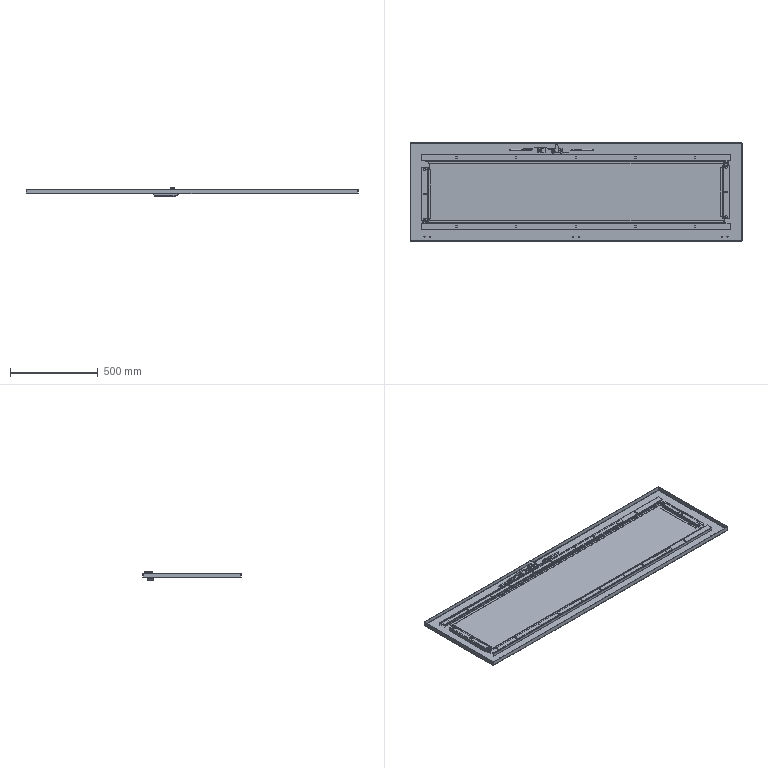Part | SolidWorks | 15 solids | 624 faces | box 1891 x 561 x 53 mm | volume 5274116 mm3 | plane 424 | cylinder 196 | cone 4 | commonest cylinder face diameters 5.2 x32 7 x32 2 x24 5 x20 6 x18 6.5 x16